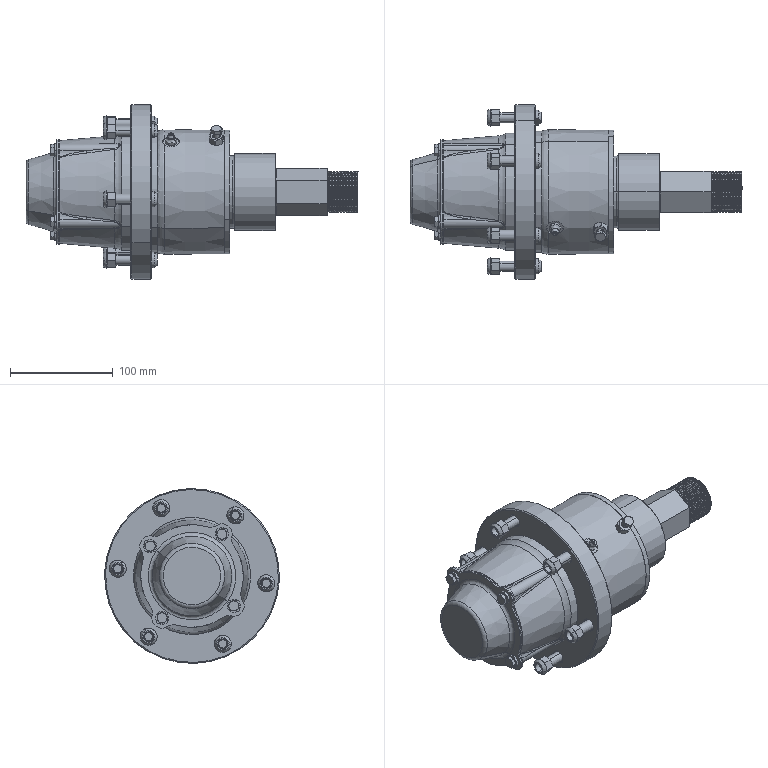Part | SolidWorks | features ReferencePattern 26, LocalCirPattern 3, CompositeCurve 1 | 84 solids | 3894 faces | volume 1867736 mm3 | plane 2462 | cylinder 812 | cone 391 | torus 150 | spline 77 | sphere 2 | commonest cylinder face diameters 9.6 x288 1 x66 10 x54 40 x45 20 x34 30 x33